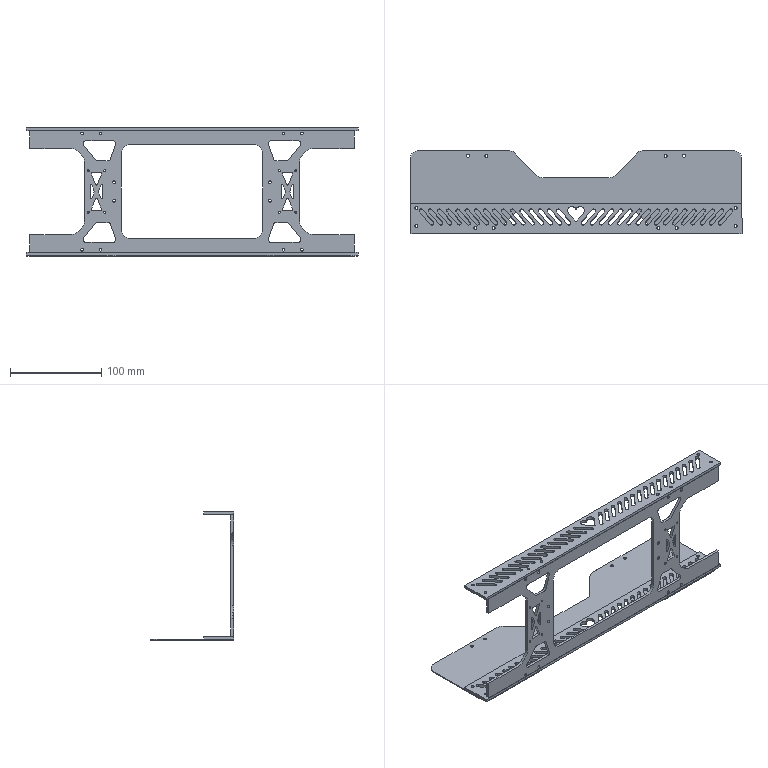Part | SolidWorks | features ICE 5, Fillet 2, Extrusion 1, MirrorSolid 1 | 4 solids | 588 faces | box 363 x 91.15 x 140 mm | volume 130923 mm3 | cylinder 368 | plane 220 | commonest cylinder face diameters 4 x192 3.2 x80 2 x30 20 x24 2.2 x16 6 x16